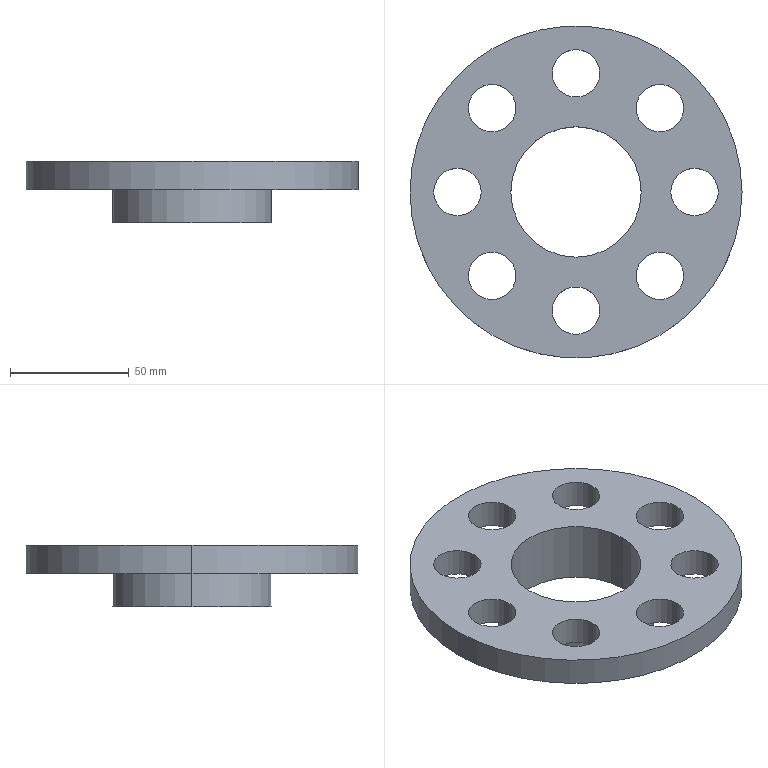Part | SolidWorks | features CirPattern 1, Cut 1, Extrusion 1, ICE 1 | 1 solid | 25 faces | box 140 x 140 x 26 mm | volume 142154 mm3 | cylinder 22 | plane 3 | commonest cylinder face diameters 20 x16 55 x2 67 x2 140 x2
STEP:
#1=CARTESIAN_POINT('',(-33.5,0.,-14.));
#2=VERTEX_POINT('',#1);
#3=CARTESIAN_POINT('',(33.5,0.,-14.));
#4=VERTEX_POINT('',#3);
#5=CARTESIAN_POINT('',(0.,0.,-14.));
#6=DIRECTION('',(0.,0.,-1.));
#7=DIRECTION('',(-1.,0.,0.));
#8=AXIS2_PLACEMENT_3D('',#5,#6,#7);
#9=CIRCLE('',#8,33.5);
#10=EDGE_CURVE('',#2,#4,#9,.T.);
#11=ORIENTED_EDGE('',*,*,#10,.F.);
#12=CARTESIAN_POINT('',(-33.5,0.,0.));
#13=VERTEX_POINT('',#12);
#14=CARTESIAN_POINT('',(-33.5,0.,-14.));
#15=DIRECTION('',(0.,0.,1.));
#16=VECTOR('',#15,1000.);
#17=LINE('',#14,#16);
#18=EDGE_CURVE('',#2,#13,#17,.T.);
#19=ORIENTED_EDGE('',*,*,#18,.T.);
#20=CARTESIAN_POINT('',(33.5,0.,0.));
#21=VERTEX_POINT('',#20);
#22=CARTESIAN_POINT('',(0.,0.,0.));
#23=DIRECTION('',(0.,0.,-1.));
#24=DIRECTION('',(1.,0.,0.));
#25=AXIS2_PLACEMENT_3D('',#22,#23,#24);
#26=CIRCLE('',#25,33.5);
#27=EDGE_CURVE('',#13,#21,#26,.T.);
#28=ORIENTED_EDGE('',*,*,#27,.T.);
#29=CARTESIAN_POINT('',(33.5,0.,-14.));
#30=DIRECTION('',(0.,0.,1.));
#31=VECTOR('',#30,1000.);
#32=LINE('',#29,#31);
#33=EDGE_CURVE('',#4,#21,#32,.T.);
#34=ORIENTED_EDGE('',*,*,#33,.F.);
#35=EDGE_LOOP('',(#11,#19,#28,#34));
#36=FACE_OUTER_BOUND('',#35,.T.);
#37=CARTESIAN_POINT('',(0.,0.,-14.));
#38=DIRECTION('',(0.,0.,1.));
#39=DIRECTION('',(1.,0.,0.));
#40=AXIS2_PLACEMENT_3D('',#37,#38,#39);
#41=CYLINDRICAL_SURFACE('',#40,33.5);
#42=ADVANCED_FACE('',(#36),#41,.T.);
#43=CARTESIAN_POINT('',(40.,0.,0.));
#44=VERTEX_POINT('',#43);
#45=CARTESIAN_POINT('',(60.,0.,0.));
#46=VERTEX_POINT('',#45);
#47=CARTESIAN_POINT('',(50.,0.,0.));
#48=DIRECTION('',(0.,0.,1.));
#49=DIRECTION('',(0.,1.,0.));
#50=AXIS2_PLACEMENT_3D('',#47,#48,#49);
#51=CIRCLE('',#50,10.);
#52=EDGE_CURVE('',#44,#46,#51,.T.);
#53=ORIENTED_EDGE('',*,*,#52,.F.);
#54=CARTESIAN_POINT('',(40.,0.,12.));
#55=VERTEX_POINT('',#54);
#56=CARTESIAN_POINT('',(40.,0.,0.));
#57=DIRECTION('',(0.,0.,1.));
#58=VECTOR('',#57,1000.);
#59=LINE('',#56,#58);
#60=EDGE_CURVE('',#44,#55,#59,.T.);
#61=ORIENTED_EDGE('',*,*,#60,.T.);
#62=CARTESIAN_POINT('',(60.,0.,12.));
#63=VERTEX_POINT('',#62);
#64=CARTESIAN_POINT('',(50.,0.,12.));
#65=DIRECTION('',(0.,0.,1.));
#66=DIRECTION('',(1.,0.,0.));
#67=AXIS2_PLACEMENT_3D('',#64,#65,#66);
#68=CIRCLE('',#67,10.);
#69=EDGE_CURVE('',#55,#63,#68,.T.);
#70=ORIENTED_EDGE('',*,*,#69,.T.);
#71=CARTESIAN_POINT('',(60.,0.,0.));
#72=DIRECTION('',(0.,0.,1.));
#73=VECTOR('',#72,1000.);
#74=LINE('',#71,#73);
#75=EDGE_CURVE('',#46,#63,#74,.T.);
#76=ORIENTED_EDGE('',*,*,#75,.F.);
#77=EDGE_LOOP('',(#53,#61,#70,#76));
#78=FACE_OUTER_BOUND('',#77,.T.);
#79=CARTESIAN_POINT('',(50.,0.,0.));
#80=DIRECTION('',(0.,0.,1.));
#81=DIRECTION('',(1.,0.,0.));
#82=AXIS2_PLACEMENT_3D('',#79,#80,#81);
#83=CYLINDRICAL_SURFACE('',#82,10.);
#84=ADVANCED_FACE('',(#78),#83,.F.);
#85=CARTESIAN_POINT('',(25.355,35.355,0.));
#86=VERTEX_POINT('',#85);
#87=CARTESIAN_POINT('',(45.355,35.355,0.));
#88=VERTEX_POINT('',#87);
#89=CARTESIAN_POINT('',(35.355,35.355,0.));
#90=DIRECTION('',(0.,0.,1.));
#91=DIRECTION('',(-0.7071,0.7071,0.));
#92=AXIS2_PLACEMENT_3D('',#89,#90,#91);
#93=CIRCLE('',#92,10.);
#94=EDGE_CURVE('',#86,#88,#93,.T.);
#95=ORIENTED_EDGE('',*,*,#94,.F.);
#96=CARTESIAN_POINT('',(25.355,35.355,12.));
#97=VERTEX_POINT('',#96);
#98=CARTESIAN_POINT('',(25.355,35.355,0.));
#99=DIRECTION('',(0.,0.,1.));
#100=VECTOR('',#99,1000.);
#101=LINE('',#98,#100);
#102=EDGE_CURVE('',#86,#97,#101,.T.);
#103=ORIENTED_EDGE('',*,*,#102,.T.);
#104=CARTESIAN_POINT('',(45.355,35.355,12.));
#105=VERTEX_POINT('',#104);
#106=CARTESIAN_POINT('',(35.355,35.355,12.));
#107=DIRECTION('',(0.,0.,1.));
#108=DIRECTION('',(1.,0.,0.));
#109=AXIS2_PLACEMENT_3D('',#106,#107,#108);
#110=CIRCLE('',#109,10.);
#111=EDGE_CURVE('',#97,#105,#110,.T.);
#112=ORIENTED_EDGE('',*,*,#111,.T.);
#113=CARTESIAN_POINT('',(45.355,35.355,0.));
#114=DIRECTION('',(0.,0.,1.));
#115=VECTOR('',#114,1000.);
#116=LINE('',#113,#115);
#117=EDGE_CURVE('',#88,#105,#116,.T.);
#118=ORIENTED_EDGE('',*,*,#117,.F.);
#119=EDGE_LOOP('',(#95,#103,#112,#118));
#120=FACE_OUTER_BOUND('',#119,.T.);
#121=CARTESIAN_POINT('',(35.355,35.355,0.));
#122=DIRECTION('',(0.,0.,1.));
#123=DIRECTION('',(1.,0.,0.));
#124=AXIS2_PLACEMENT_3D('',#121,#122,#123);
#125=CYLINDRICAL_SURFACE('',#124,10.);
#126=ADVANCED_FACE('',(#120),#125,.F.);
#127=CARTESIAN_POINT('',(-10.,50.,0.));
#128=VERTEX_POINT('',#127);
#129=CARTESIAN_POINT('',(10.,50.,0.));
#130=VERTEX_POINT('',#129);
#131=CARTESIAN_POINT('',(0.,50.,0.));
#132=DIRECTION('',(0.,0.,1.));
#133=DIRECTION('',(-1.,0.,0.));
#134=AXIS2_PLACEMENT_3D('',#131,#132,#133);
#135=CIRCLE('',#134,10.);
#136=EDGE_CURVE('',#128,#130,#135,.T.);
#137=ORIENTED_EDGE('',*,*,#136,.F.);
#138=CARTESIAN_POINT('',(-10.,50.,12.));
#139=VERTEX_POINT('',#138);
#140=CARTESIAN_POINT('',(-10.,50.,0.));
#141=DIRECTION('',(0.,0.,1.));
#142=VECTOR('',#141,1000.);
#143=LINE('',#140,#142);
#144=EDGE_CURVE('',#128,#139,#143,.T.);
#145=ORIENTED_EDGE('',*,*,#144,.T.);
#146=CARTESIAN_POINT('',(10.,50.,12.));
#147=VERTEX_POINT('',#146);
#148=CARTESIAN_POINT('',(0.,50.,12.));
#149=DIRECTION('',(0.,0.,1.));
#150=DIRECTION('',(1.,0.,0.));
#151=AXIS2_PLACEMENT_3D('',#148,#149,#150);
#152=CIRCLE('',#151,10.);
#153=EDGE_CURVE('',#139,#147,#152,.T.);
#154=ORIENTED_EDGE('',*,*,#153,.T.);
#155=CARTESIAN_POINT('',(10.,50.,0.));
#156=DIRECTION('',(0.,0.,1.));
#157=VECTOR('',#156,1000.);
#158=LINE('',#155,#157);
#159=EDGE_CURVE('',#130,#147,#158,.T.);
#160=ORIENTED_EDGE('',*,*,#159,.F.);
#161=EDGE_LOOP('',(#137,#145,#154,#160));
#162=FACE_OUTER_BOUND('',#161,.T.);
#163=CARTESIAN_POINT('',(0.,50.,0.));
#164=DIRECTION('',(0.,0.,1.));
#165=DIRECTION('',(1.,0.,0.));
#166=AXIS2_PLACEMENT_3D('',#163,#164,#165);
#167=CYLINDRICAL_SURFACE('',#166,10.);
#168=ADVANCED_FACE('',(#162),#167,.F.);
#169=CARTESIAN_POINT('',(-45.355,35.355,0.));
#170=VERTEX_POINT('',#169);
#171=CARTESIAN_POINT('',(-25.355,35.355,0.));
#172=VERTEX_POINT('',#171);
#173=CARTESIAN_POINT('',(-35.355,35.355,0.));
#174=DIRECTION('',(0.,0.,1.));
#175=DIRECTION('',(-0.7071,-0.7071,0.));
#176=AXIS2_PLACEMENT_3D('',#173,#174,#175);
#177=CIRCLE('',#176,10.);
#178=EDGE_CURVE('',#170,#172,#177,.T.);
#179=ORIENTED_EDGE('',*,*,#178,.F.);
#180=CARTESIAN_POINT('',(-45.355,35.355,12.));
#181=VERTEX_POINT('',#180);
#182=CARTESIAN_POINT('',(-45.355,35.355,0.));
#183=DIRECTION('',(0.,0.,1.));
#184=VECTOR('',#183,1000.);
#185=LINE('',#182,#184);
#186=EDGE_CURVE('',#170,#181,#185,.T.);
#187=ORIENTED_EDGE('',*,*,#186,.T.);
#188=CARTESIAN_POINT('',(-25.355,35.355,12.));
#189=VERTEX_POINT('',#188);
#190=CARTESIAN_POINT('',(-35.355,35.355,12.));
#191=DIRECTION('',(0.,0.,1.));
#192=DIRECTION('',(1.,0.,0.));
#193=AXIS2_PLACEMENT_3D('',#190,#191,#192);
#194=CIRCLE('',#193,10.);
#195=EDGE_CURVE('',#181,#189,#194,.T.);
#196=ORIENTED_EDGE('',*,*,#195,.T.);
#197=CARTESIAN_POINT('',(-25.355,35.355,0.));
#198=DIRECTION('',(0.,0.,1.));
#199=VECTOR('',#198,1000.);
#200=LINE('',#197,#199);
#201=EDGE_CURVE('',#172,#189,#200,.T.);
#202=ORIENTED_EDGE('',*,*,#201,.F.);
#203=EDGE_LOOP('',(#179,#187,#196,#202));
#204=FACE_OUTER_BOUND('',#203,.T.);
#205=CARTESIAN_POINT('',(-35.355,35.355,0.));
#206=DIRECTION('',(0.,0.,1.));
#207=DIRECTION('',(1.,0.,0.));
#208=AXIS2_PLACEMENT_3D('',#205,#206,#207);
#209=CYLINDRICAL_SURFACE('',#208,10.);
#210=ADVANCED_FACE('',(#204),#209,.F.);
#211=CARTESIAN_POINT('',(-60.,0.,0.));
#212=VERTEX_POINT('',#211);
#213=CARTESIAN_POINT('',(-40.,0.,0.));
#214=VERTEX_POINT('',#213);
#215=CARTESIAN_POINT('',(-50.,0.,0.));
#216=DIRECTION('',(0.,0.,1.));
#217=DIRECTION('',(0.,-1.,0.));
#218=AXIS2_PLACEMENT_3D('',#215,#216,#217);
#219=CIRCLE('',#218,10.);
#220=EDGE_CURVE('',#212,#214,#219,.T.);
#221=ORIENTED_EDGE('',*,*,#220,.F.);
#222=CARTESIAN_POINT('',(-60.,0.,12.));
#223=VERTEX_POINT('',#222);
#224=CARTESIAN_POINT('',(-60.,0.,0.));
#225=DIRECTION('',(0.,0.,1.));
#226=VECTOR('',#225,1000.);
#227=LINE('',#224,#226);
#228=EDGE_CURVE('',#212,#223,#227,.T.);
#229=ORIENTED_EDGE('',*,*,#228,.T.);
#230=CARTESIAN_POINT('',(-40.,0.,12.));
#231=VERTEX_POINT('',#230);
#232=CARTESIAN_POINT('',(-50.,0.,12.));
#233=DIRECTION('',(0.,0.,1.));
#234=DIRECTION('',(1.,0.,0.));
#235=AXIS2_PLACEMENT_3D('',#232,#233,#234);
#236=CIRCLE('',#235,10.);
#237=EDGE_CURVE('',#223,#231,#236,.T.);
#238=ORIENTED_EDGE('',*,*,#237,.T.);
#239=CARTESIAN_POINT('',(-40.,0.,0.));
#240=DIRECTION('',(0.,0.,1.));
#241=VECTOR('',#240,1000.);
#242=LINE('',#239,#241);
#243=EDGE_CURVE('',#214,#231,#242,.T.);
#244=ORIENTED_EDGE('',*,*,#243,.F.);
#245=EDGE_LOOP('',(#221,#229,#238,#244));
#246=FACE_OUTER_BOUND('',#245,.T.);
#247=CARTESIAN_POINT('',(-50.,0.,0.));
#248=DIRECTION('',(0.,0.,1.));
#249=DIRECTION('',(1.,0.,0.));
#250=AXIS2_PLACEMENT_3D('',#247,#248,#249);
#251=CYLINDRICAL_SURFACE('',#250,10.);
#252=ADVANCED_FACE('',(#246),#251,.F.);
#253=CARTESIAN_POINT('',(-45.355,-35.355,0.));
#254=VERTEX_POINT('',#253);
#255=CARTESIAN_POINT('',(-25.355,-35.355,0.));
#256=VERTEX_POINT('',#255);
#257=CARTESIAN_POINT('',(-35.355,-35.355,0.));
#258=DIRECTION('',(0.,0.,1.));
#259=DIRECTION('',(0.7071,-0.7071,0.));
#260=AXIS2_PLACEMENT_3D('',#257,#258,#259);
#261=CIRCLE('',#260,10.);
#262=EDGE_CURVE('',#254,#256,#261,.T.);
#263=ORIENTED_EDGE('',*,*,#262,.F.);
#264=CARTESIAN_POINT('',(-45.355,-35.355,12.));
#265=VERTEX_POINT('',#264);
#266=CARTESIAN_POINT('',(-45.355,-35.355,0.));
#267=DIRECTION('',(0.,0.,1.));
#268=VECTOR('',#267,1000.);
#269=LINE('',#266,#268);
#270=EDGE_CURVE('',#254,#265,#269,.T.);
#271=ORIENTED_EDGE('',*,*,#270,.T.);
#272=CARTESIAN_POINT('',(-25.355,-35.355,12.));
#273=VERTEX_POINT('',#272);
#274=CARTESIAN_POINT('',(-35.355,-35.355,12.));
#275=DIRECTION('',(0.,0.,1.));
#276=DIRECTION('',(1.,0.,0.));
#277=AXIS2_PLACEMENT_3D('',#274,#275,#276);
#278=CIRCLE('',#277,10.);
#279=EDGE_CURVE('',#265,#273,#278,.T.);
#280=ORIENTED_EDGE('',*,*,#279,.T.);
#281=CARTESIAN_POINT('',(-25.355,-35.355,0.));
#282=DIRECTION('',(0.,0.,1.));
#283=VECTOR('',#282,1000.);
#284=LINE('',#281,#283);
#285=EDGE_CURVE('',#256,#273,#284,.T.);
#286=ORIENTED_EDGE('',*,*,#285,.F.);
#287=EDGE_LOOP('',(#263,#271,#280,#286));
#288=FACE_OUTER_BOUND('',#287,.T.);
#289=CARTESIAN_POINT('',(-35.355,-35.355,0.));
#290=DIRECTION('',(0.,0.,1.));
#291=DIRECTION('',(1.,0.,0.));
#292=AXIS2_PLACEMENT_3D('',#289,#290,#291);
#293=CYLINDRICAL_SURFACE('',#292,10.);
#294=ADVANCED_FACE('',(#288),#293,.F.);
#295=CARTESIAN_POINT('',(25.355,-35.355,0.));
#296=VERTEX_POINT('',#295);
#297=CARTESIAN_POINT('',(45.355,-35.355,0.));
#298=VERTEX_POINT('',#297);
#299=CARTESIAN_POINT('',(35.355,-35.355,0.));
#300=DIRECTION('',(0.,0.,1.));
#301=DIRECTION('',(0.7071,0.7071,0.));
#302=AXIS2_PLACEMENT_3D('',#299,#300,#301);
#303=CIRCLE('',#302,10.);
#304=EDGE_CURVE('',#296,#298,#303,.T.);
#305=ORIENTED_EDGE('',*,*,#304,.F.);
#306=CARTESIAN_POINT('',(25.355,-35.355,12.));
#307=VERTEX_POINT('',#306);
#308=CARTESIAN_POINT('',(25.355,-35.355,0.));
#309=DIRECTION('',(0.,0.,1.));
#310=VECTOR('',#309,1000.);
#311=LINE('',#308,#310);
#312=EDGE_CURVE('',#296,#307,#311,.T.);
#313=ORIENTED_EDGE('',*,*,#312,.T.);
#314=CARTESIAN_POINT('',(45.355,-35.355,12.));
#315=VERTEX_POINT('',#314);
#316=CARTESIAN_POINT('',(35.355,-35.355,12.));
#317=DIRECTION('',(0.,0.,1.));
#318=DIRECTION('',(1.,0.,0.));
#319=AXIS2_PLACEMENT_3D('',#316,#317,#318);
#320=CIRCLE('',#319,10.);
#321=EDGE_CURVE('',#307,#315,#320,.T.);
#322=ORIENTED_EDGE('',*,*,#321,.T.);
#323=CARTESIAN_POINT('',(45.355,-35.355,0.));
#324=DIRECTION('',(0.,0.,1.));
#325=VECTOR('',#324,1000.);
#326=LINE('',#323,#325);
#327=EDGE_CURVE('',#298,#315,#326,.T.);
#328=ORIENTED_EDGE('',*,*,#327,.F.);
#329=EDGE_LOOP('',(#305,#313,#322,#328));
#330=FACE_OUTER_BOUND('',#329,.T.);
#331=CARTESIAN_POINT('',(35.355,-35.355,0.));
#332=DIRECTION('',(0.,0.,1.));
#333=DIRECTION('',(1.,0.,0.));
#334=AXIS2_PLACEMENT_3D('',#331,#332,#333);
#335=CYLINDRICAL_SURFACE('',#334,10.);
#336=ADVANCED_FACE('',(#330),#335,.F.);
#337=CARTESIAN_POINT('',(-10.,-50.,0.));
#338=VERTEX_POINT('',#337);
#339=CARTESIAN_POINT('',(10.,-50.,0.));
#340=VERTEX_POINT('',#339);
#341=CARTESIAN_POINT('',(0.,-50.,0.));
#342=DIRECTION('',(0.,0.,1.));
#343=DIRECTION('',(1.,0.,0.));
#344=AXIS2_PLACEMENT_3D('',#341,#342,#343);
#345=CIRCLE('',#344,10.);
#346=EDGE_CURVE('',#338,#340,#345,.T.);
#347=ORIENTED_EDGE('',*,*,#346,.F.);
#348=CARTESIAN_POINT('',(-10.,-50.,12.));
#349=VERTEX_POINT('',#348);
#350=CARTESIAN_POINT('',(-10.,-50.,0.));
#351=DIRECTION('',(0.,0.,1.));
#352=VECTOR('',#351,1000.);
#353=LINE('',#350,#352);
#354=EDGE_CURVE('',#338,#349,#353,.T.);
#355=ORIENTED_EDGE('',*,*,#354,.T.);
#356=CARTESIAN_POINT('',(10.,-50.,12.));
#357=VERTEX_POINT('',#356);
#358=CARTESIAN_POINT('',(0.,-50.,12.));
#359=DIRECTION('',(0.,0.,1.));
#360=DIRECTION('',(1.,0.,0.));
#361=AXIS2_PLACEMENT_3D('',#358,#359,#360);
#362=CIRCLE('',#361,10.);
#363=EDGE_CURVE('',#349,#357,#362,.T.);
#364=ORIENTED_EDGE('',*,*,#363,.T.);
#365=CARTESIAN_POINT('',(10.,-50.,0.));
#366=DIRECTION('',(0.,0.,1.));
#367=VECTOR('',#366,1000.);
#368=LINE('',#365,#367);
#369=EDGE_CURVE('',#340,#357,#368,.T.);
#370=ORIENTED_EDGE('',*,*,#369,.F.);
#371=EDGE_LOOP('',(#347,#355,#364,#370));
#372=FACE_OUTER_BOUND('',#371,.T.);
#373=CARTESIAN_POINT('',(0.,-50.,0.));
#374=DIRECTION('',(0.,0.,1.));
#375=DIRECTION('',(1.,0.,0.));
#376=AXIS2_PLACEMENT_3D('',#373,#374,#375);
#377=CYLINDRICAL_SURFACE('',#376,10.);
#378=ADVANCED_FACE('',(#372),#377,.F.);
#379=CARTESIAN_POINT('',(-27.5,0.,12.));
#380=VERTEX_POINT('',#379);
#381=CARTESIAN_POINT('',(27.5,0.,12.));
#382=VERTEX_POINT('',#381);
#383=CARTESIAN_POINT('',(0.,0.,12.));
#384=DIRECTION('',(0.,0.,1.));
#385=DIRECTION('',(1.,0.,0.));
#386=AXIS2_PLACEMENT_3D('',#383,#384,#385);
#387=CIRCLE('',#386,27.5);
#388=EDGE_CURVE('',#380,#382,#387,.T.);
#389=ORIENTED_EDGE('',*,*,#388,.T.);
#390=CARTESIAN_POINT('',(27.5,0.,-14.));
#391=VERTEX_POINT('',#390);
#392=CARTESIAN_POINT('',(27.5,0.,12.));
#393=DIRECTION('',(0.,0.,-1.));
#394=VECTOR('',#393,1000.);
#395=LINE('',#392,#394);
#396=EDGE_CURVE('',#382,#391,#395,.T.);
#397=ORIENTED_EDGE('',*,*,#396,.T.);
#398=CARTESIAN_POINT('',(-27.5,0.,-14.));
#399=VERTEX_POINT('',#398);
#400=CARTESIAN_POINT('',(0.,0.,-14.));
#401=DIRECTION('',(0.,0.,-1.));
#402=DIRECTION('',(-1.,0.,0.));
#403=AXIS2_PLACEMENT_3D('',#400,#401,#402);
#404=CIRCLE('',#403,27.5);
#405=EDGE_CURVE('',#391,#399,#404,.T.);
#406=ORIENTED_EDGE('',*,*,#405,.T.);
#407=CARTESIAN_POINT('',(-27.5,0.,12.));
#408=DIRECTION('',(0.,0.,-1.));
#409=VECTOR('',#408,1000.);
#410=LINE('',#407,#409);
#411=EDGE_CURVE('',#380,#399,#410,.T.);
#412=ORIENTED_EDGE('',*,*,#411,.F.);
#413=EDGE_LOOP('',(#389,#397,#406,#412));
#414=FACE_OUTER_BOUND('',#413,.T.);
#415=CARTESIAN_POINT('',(0.,0.,12.));
#416=DIRECTION('',(0.,0.,-1.));
#417=DIRECTION('',(-1.,0.,0.));
#418=AXIS2_PLACEMENT_3D('',#415,#416,#417);
#419=CYLINDRICAL_SURFACE('',#418,27.5);
#420=ADVANCED_FACE('',(#414),#419,.F.);
#421=CARTESIAN_POINT('',(70.,0.,12.));
#422=VERTEX_POINT('',#421);
#423=CARTESIAN_POINT('',(-70.,0.,12.));
#424=VERTEX_POINT('',#423);
#425=CARTESIAN_POINT('',(0.,0.,12.));
#426=DIRECTION('',(0.,0.,1.));
#427=DIRECTION('',(1.,0.,0.));
#428=AXIS2_PLACEMENT_3D('',#425,#426,#427);
#429=CIRCLE('',#428,70.);
#430=EDGE_CURVE('',#422,#424,#429,.T.);
#431=ORIENTED_EDGE('',*,*,#430,.F.);
#432=CARTESIAN_POINT('',(70.,0.,0.));
#433=VERTEX_POINT('',#432);
#434=CARTESIAN_POINT('',(70.,0.,12.));
#435=DIRECTION('',(0.,0.,-1.));
#436=VECTOR('',#435,1000.);
#437=LINE('',#434,#436);
#438=EDGE_CURVE('',#422,#433,#437,.T.);
#439=ORIENTED_EDGE('',*,*,#438,.T.);
#440=CARTESIAN_POINT('',(-70.,0.,0.));
#441=VERTEX_POINT('',#440);
#442=CARTESIAN_POINT('',(0.,0.,0.));
#443=DIRECTION('',(0.,0.,1.));
#444=DIRECTION('',(1.,0.,0.));
#445=AXIS2_PLACEMENT_3D('',#442,#443,#444);
#446=CIRCLE('',#445,70.);
#447=EDGE_CURVE('',#433,#441,#446,.T.);
#448=ORIENTED_EDGE('',*,*,#447,.T.);
#449=CARTESIAN_POINT('',(-70.,0.,12.));
#450=DIRECTION('',(0.,0.,-1.));
#451=VECTOR('',#450,1000.);
#452=LINE('',#449,#451);
#453=EDGE_CURVE('',#424,#441,#452,.T.);
#454=ORIENTED_EDGE('',*,*,#453,.F.);
#455=EDGE_LOOP('',(#431,#439,#448,#454));
#456=FACE_OUTER_BOUND('',#455,.T.);
#457=CARTESIAN_POINT('',(0.,0.,12.));
#458=DIRECTION('',(0.,0.,-1.));
#459=DIRECTION('',(-1.,0.,0.));
#460=AXIS2_PLACEMENT_3D('',#457,#458,#459);
#461=CYLINDRICAL_SURFACE('',#460,70.);
#462=ADVANCED_FACE('',(#456),#461,.T.);
#463=CARTESIAN_POINT('',(0.,0.,0.));
#464=DIRECTION('',(0.,0.,1.));
#465=DIRECTION('',(1.,0.,0.));
#466=AXIS2_PLACEMENT_3D('',#463,#464,#465);
#467=CIRCLE('',#466,70.);
#468=EDGE_CURVE('',#441,#433,#467,.T.);
#469=ORIENTED_EDGE('',*,*,#468,.F.);
#470=ORIENTED_EDGE('',*,*,#447,.F.);
#471=EDGE_LOOP('',(#469,#470));
#472=FACE_OUTER_BOUND('',#471,.T.);
#473=CARTESIAN_POINT('',(0.,-50.,0.));
#474=DIRECTION('',(0.,0.,1.));
#475=DIRECTION('',(1.,0.,0.));
#476=AXIS2_PLACEMENT_3D('',#473,#474,#475);
#477=CIRCLE('',#476,10.);
#478=EDGE_CURVE('',#340,#338,#477,.T.);
#479=ORIENTED_EDGE('',*,*,#478,.T.);
#480=ORIENTED_EDGE('',*,*,#346,.T.);
#481=EDGE_LOOP('',(#479,#480));
#482=FACE_BOUND('',#481,.T.);
#483=CARTESIAN_POINT('',(35.355,-35.355,0.));
#484=DIRECTION('',(0.,0.,1.));
#485=DIRECTION('',(0.7071,0.7071,0.));
#486=AXIS2_PLACEMENT_3D('',#483,#484,#485);
#487=CIRCLE('',#486,10.);
#488=EDGE_CURVE('',#298,#296,#487,.T.);
#489=ORIENTED_EDGE('',*,*,#488,.T.);
#490=ORIENTED_EDGE('',*,*,#304,.T.);
#491=EDGE_LOOP('',(#489,#490));
#492=FACE_BOUND('',#491,.T.);
#493=CARTESIAN_POINT('',(-35.355,-35.355,0.));
#494=DIRECTION('',(0.,0.,1.));
#495=DIRECTION('',(0.7071,-0.7071,0.));
#496=AXIS2_PLACEMENT_3D('',#493,#494,#495);
#497=CIRCLE('',#496,10.);
#498=EDGE_CURVE('',#256,#254,#497,.T.);
#499=ORIENTED_EDGE('',*,*,#498,.T.);
#500=ORIENTED_EDGE('',*,*,#262,.T.);
#501=EDGE_LOOP('',(#499,#500));
#502=FACE_BOUND('',#501,.T.);
#503=CARTESIAN_POINT('',(-50.,0.,0.));
#504=DIRECTION('',(0.,0.,1.));
#505=DIRECTION('',(0.,-1.,0.));
#506=AXIS2_PLACEMENT_3D('',#503,#504,#505);
#507=CIRCLE('',#506,10.);
#508=EDGE_CURVE('',#214,#212,#507,.T.);
#509=ORIENTED_EDGE('',*,*,#508,.T.);
#510=ORIENTED_EDGE('',*,*,#220,.T.);
#511=EDGE_LOOP('',(#509,#510));
#512=FACE_BOUND('',#511,.T.);
#513=CARTESIAN_POINT('',(-35.355,35.355,0.));
#514=DIRECTION('',(0.,0.,1.));
#515=DIRECTION('',(-0.7071,-0.7071,0.));
#516=AXIS2_PLACEMENT_3D('',#513,#514,#515);
#517=CIRCLE('',#516,10.);
#518=EDGE_CURVE('',#172,#170,#517,.T.);
#519=ORIENTED_EDGE('',*,*,#518,.T.);
#520=ORIENTED_EDGE('',*,*,#178,.T.);
#521=EDGE_LOOP('',(#519,#520));
#522=FACE_BOUND('',#521,.T.);
#523=CARTESIAN_POINT('',(0.,50.,0.));
#524=DIRECTION('',(0.,0.,1.));
#525=DIRECTION('',(-1.,0.,0.));
#526=AXIS2_PLACEMENT_3D('',#523,#524,#525);
#527=CIRCLE('',#526,10.);
#528=EDGE_CURVE('',#130,#128,#527,.T.);
#529=ORIENTED_EDGE('',*,*,#528,.T.);
#530=ORIENTED_EDGE('',*,*,#136,.T.);
#531=EDGE_LOOP('',(#529,#530));
#532=FACE_BOUND('',#531,.T.);
#533=CARTESIAN_POINT('',(35.355,35.355,0.));
#534=DIRECTION('',(0.,0.,1.));
#535=DIRECTION('',(-0.7071,0.7071,0.));
#536=AXIS2_PLACEMENT_3D('',#533,#534,#535);
#537=CIRCLE('',#536,10.);
#538=EDGE_CURVE('',#88,#86,#537,.T.);
#539=ORIENTED_EDGE('',*,*,#538,.T.);
#540=ORIENTED_EDGE('',*,*,#94,.T.);
#541=EDGE_LOOP('',(#539,#540));
#542=FACE_BOUND('',#541,.T.);
#543=CARTESIAN_POINT('',(50.,0.,0.));
#544=DIRECTION('',(0.,0.,1.));
#545=DIRECTION('',(0.,1.,0.));
#546=AXIS2_PLACEMENT_3D('',#543,#544,#545);
#547=CIRCLE('',#546,10.);
#548=EDGE_CURVE('',#46,#44,#547,.T.);
#549=ORIENTED_EDGE('',*,*,#548,.T.);
#550=ORIENTED_EDGE('',*,*,#52,.T.);
#551=EDGE_LOOP('',(#549,#550));
#552=FACE_BOUND('',#551,.T.);
#553=CARTESIAN_POINT('',(0.,0.,0.));
#554=DIRECTION('',(0.,0.,-1.));
#555=DIRECTION('',(1.,0.,0.));
#556=AXIS2_PLACEMENT_3D('',#553,#554,#555);
#557=CIRCLE('',#556,33.5);
#558=EDGE_CURVE('',#21,#13,#557,.T.);
#559=ORIENTED_EDGE('',*,*,#558,.F.);
#560=ORIENTED_EDGE('',*,*,#27,.F.);
#561=EDGE_LOOP('',(#559,#560));
#562=FACE_BOUND('',#561,.T.);
#563=CARTESIAN_POINT('',(0.,0.,0.));
#564=DIRECTION('',(0.,0.,1.));
#565=DIRECTION('',(1.,0.,0.));
#566=AXIS2_PLACEMENT_3D('',#563,#564,#565);
#567=PLANE('',#566);
#568=ADVANCED_FACE('',(#472,#482,#492,#502,#512,#522,#532,#542,#552,#562),#567,.F.);
#569=CARTESIAN_POINT('',(50.,0.,12.));
#570=DIRECTION('',(0.,0.,1.));
#571=DIRECTION('',(1.,0.,0.));
#572=AXIS2_PLACEMENT_3D('',#569,#570,#571);
#573=CIRCLE('',#572,10.);
#574=EDGE_CURVE('',#63,#55,#573,.T.);
#575=ORIENTED_EDGE('',*,*,#574,.F.);
#576=ORIENTED_EDGE('',*,*,#69,.F.);
#577=EDGE_LOOP('',(#575,#576));
#578=FACE_BOUND('',#577,.T.);
#579=CARTESIAN_POINT('',(35.355,35.355,12.));
#580=DIRECTION('',(0.,0.,1.));
#581=DIRECTION('',(1.,0.,0.));
#582=AXIS2_PLACEMENT_3D('',#579,#580,#581);
#583=CIRCLE('',#582,10.);
#584=EDGE_CURVE('',#105,#97,#583,.T.);
#585=ORIENTED_EDGE('',*,*,#584,.F.);
#586=ORIENTED_EDGE('',*,*,#111,.F.);
#587=EDGE_LOOP('',(#585,#586));
#588=FACE_BOUND('',#587,.T.);
#589=CARTESIAN_POINT('',(0.,50.,12.));
#590=DIRECTION('',(0.,0.,1.));
#591=DIRECTION('',(1.,0.,0.));
#592=AXIS2_PLACEMENT_3D('',#589,#590,#591);
#593=CIRCLE('',#592,10.);
#594=EDGE_CURVE('',#147,#139,#593,.T.);
#595=ORIENTED_EDGE('',*,*,#594,.F.);
#596=ORIENTED_EDGE('',*,*,#153,.F.);
#597=EDGE_LOOP('',(#595,#596));
#598=FACE_BOUND('',#597,.T.);
#599=CARTESIAN_POINT('',(-35.355,35.355,12.));
#600=DIRECTION('',(0.,0.,1.));
#601=DIRECTION('',(1.,0.,0.));
#602=AXIS2_PLACEMENT_3D('',#599,#600,#601);
#603=CIRCLE('',#602,10.);
#604=EDGE_CURVE('',#189,#181,#603,.T.);
#605=ORIENTED_EDGE('',*,*,#604,.F.);
#606=ORIENTED_EDGE('',*,*,#195,.F.);
#607=EDGE_LOOP('',(#605,#606));
#608=FACE_BOUND('',#607,.T.);
#609=CARTESIAN_POINT('',(-50.,0.,12.));
#610=DIRECTION('',(0.,0.,1.));
#611=DIRECTION('',(1.,0.,0.));
#612=AXIS2_PLACEMENT_3D('',#609,#610,#611);
#613=CIRCLE('',#612,10.);
#614=EDGE_CURVE('',#231,#223,#613,.T.);
#615=ORIENTED_EDGE('',*,*,#614,.F.);
#616=ORIENTED_EDGE('',*,*,#237,.F.);
#617=EDGE_LOOP('',(#615,#616));
#618=FACE_BOUND('',#617,.T.);
#619=CARTESIAN_POINT('',(-35.355,-35.355,12.));
#620=DIRECTION('',(0.,0.,1.));
#621=DIRECTION('',(1.,0.,0.));
#622=AXIS2_PLACEMENT_3D('',#619,#620,#621);
#623=CIRCLE('',#622,10.);
#624=EDGE_CURVE('',#273,#265,#623,.T.);
#625=ORIENTED_EDGE('',*,*,#624,.F.);
#626=ORIENTED_EDGE('',*,*,#279,.F.);
#627=EDGE_LOOP('',(#625,#626));
#628=FACE_BOUND('',#627,.T.);
#629=CARTESIAN_POINT('',(35.355,-35.355,12.));
#630=DIRECTION('',(0.,0.,1.));
#631=DIRECTION('',(1.,0.,0.));
#632=AXIS2_PLACEMENT_3D('',#629,#630,#631);
#633=CIRCLE('',#632,10.);
#634=EDGE_CURVE('',#315,#307,#633,.T.);
#635=ORIENTED_EDGE('',*,*,#634,.F.);
#636=ORIENTED_EDGE('',*,*,#321,.F.);
#637=EDGE_LOOP('',(#635,#636));
#638=FACE_BOUND('',#637,.T.);
#639=CARTESIAN_POINT('',(0.,-50.,12.));
#640=DIRECTION('',(0.,0.,1.));
#641=DIRECTION('',(1.,0.,0.));
#642=AXIS2_PLACEMENT_3D('',#639,#640,#641);
#643=CIRCLE('',#642,10.);
#644=EDGE_CURVE('',#357,#349,#643,.T.);
#645=ORIENTED_EDGE('',*,*,#644,.F.);
#646=ORIENTED_EDGE('',*,*,#363,.F.);
#647=EDGE_LOOP('',(#645,#646));
#648=FACE_BOUND('',#647,.T.);
#649=CARTESIAN_POINT('',(0.,0.,12.));
#650=DIRECTION('',(0.,0.,1.));
#651=DIRECTION('',(1.,0.,0.));
#652=AXIS2_PLACEMENT_3D('',#649,#650,#651);
#653=CIRCLE('',#652,70.);
#654=EDGE_CURVE('',#424,#422,#653,.T.);
#655=ORIENTED_EDGE('',*,*,#654,.T.);
#656=ORIENTED_EDGE('',*,*,#430,.T.);
#657=EDGE_LOOP('',(#655,#656));
#658=FACE_OUTER_BOUND('',#657,.T.);
#659=ORIENTED_EDGE('',*,*,#388,.F.);
#660=CARTESIAN_POINT('',(0.,0.,12.));
#661=DIRECTION('',(0.,0.,1.));
#662=DIRECTION('',(1.,0.,0.));
#663=AXIS2_PLACEMENT_3D('',#660,#661,#662);
#664=CIRCLE('',#663,27.5);
#665=EDGE_CURVE('',#382,#380,#664,.T.);
#666=ORIENTED_EDGE('',*,*,#665,.F.);
#667=EDGE_LOOP('',(#659,#666));
#668=FACE_BOUND('',#667,.T.);
#669=CARTESIAN_POINT('',(0.,0.,12.));
#670=DIRECTION('',(0.,0.,1.));
#671=DIRECTION('',(1.,0.,0.));
#672=AXIS2_PLACEMENT_3D('',#669,#670,#671);
#673=PLANE('',#672);
#674=ADVANCED_FACE('',(#578,#588,#598,#608,#618,#628,#638,#648,#658,#668),#673,.T.);
#675=ORIENTED_EDGE('',*,*,#438,.F.);
#676=ORIENTED_EDGE('',*,*,#654,.F.);
#677=ORIENTED_EDGE('',*,*,#453,.T.);
#678=ORIENTED_EDGE('',*,*,#468,.T.);
#679=EDGE_LOOP('',(#675,#676,#677,#678));
#680=FACE_OUTER_BOUND('',#679,.T.);
#681=CARTESIAN_POINT('',(0.,0.,12.));
#682=DIRECTION('',(0.,0.,-1.));
#683=DIRECTION('',(-1.,0.,0.));
#684=AXIS2_PLACEMENT_3D('',#681,#682,#683);
#685=CYLINDRICAL_SURFACE('',#684,70.);
#686=ADVANCED_FACE('',(#680),#685,.T.);
#687=ORIENTED_EDGE('',*,*,#396,.F.);
#688=ORIENTED_EDGE('',*,*,#665,.T.);
#689=ORIENTED_EDGE('',*,*,#411,.T.);
#690=CARTESIAN_POINT('',(0.,0.,-14.));
#691=DIRECTION('',(0.,0.,-1.));
#692=DIRECTION('',(-1.,0.,0.));
#693=AXIS2_PLACEMENT_3D('',#690,#691,#692);
#694=CIRCLE('',#693,27.5);
#695=EDGE_CURVE('',#399,#391,#694,.T.);
#696=ORIENTED_EDGE('',*,*,#695,.T.);
#697=EDGE_LOOP('',(#687,#688,#689,#696));
#698=FACE_OUTER_BOUND('',#697,.T.);
#699=CARTESIAN_POINT('',(0.,0.,12.));
#700=DIRECTION('',(0.,0.,-1.));
#701=DIRECTION('',(-1.,0.,0.));
#702=AXIS2_PLACEMENT_3D('',#699,#700,#701);
#703=CYLINDRICAL_SURFACE('',#702,27.5);
#704=ADVANCED_FACE('',(#698),#703,.F.);
#705=ORIENTED_EDGE('',*,*,#354,.F.);
#706=ORIENTED_EDGE('',*,*,#478,.F.);
#707=ORIENTED_EDGE('',*,*,#369,.T.);
#708=ORIENTED_EDGE('',*,*,#644,.T.);
#709=EDGE_LOOP('',(#705,#706,#707,#708));
#710=FACE_OUTER_BOUND('',#709,.T.);
#711=CARTESIAN_POINT('',(0.,-50.,0.));
#712=DIRECTION('',(0.,0.,1.));
#713=DIRECTION('',(1.,0.,0.));
#714=AXIS2_PLACEMENT_3D('',#711,#712,#713);
#715=CYLINDRICAL_SURFACE('',#714,10.);
#716=ADVANCED_FACE('',(#710),#715,.F.);
#717=ORIENTED_EDGE('',*,*,#312,.F.);
#718=ORIENTED_EDGE('',*,*,#488,.F.);
#719=ORIENTED_EDGE('',*,*,#327,.T.);
#720=ORIENTED_EDGE('',*,*,#634,.T.);
#721=EDGE_LOOP('',(#717,#718,#719,#720));
#722=FACE_OUTER_BOUND('',#721,.T.);
#723=CARTESIAN_POINT('',(35.355,-35.355,0.));
#724=DIRECTION('',(0.,0.,1.));
#725=DIRECTION('',(1.,0.,0.));
#726=AXIS2_PLACEMENT_3D('',#723,#724,#725);
#727=CYLINDRICAL_SURFACE('',#726,10.);
#728=ADVANCED_FACE('',(#722),#727,.F.);
#729=ORIENTED_EDGE('',*,*,#270,.F.);
#730=ORIENTED_EDGE('',*,*,#498,.F.);
#731=ORIENTED_EDGE('',*,*,#285,.T.);
#732=ORIENTED_EDGE('',*,*,#624,.T.);
#733=EDGE_LOOP('',(#729,#730,#731,#732));
#734=FACE_OUTER_BOUND('',#733,.T.);
#735=CARTESIAN_POINT('',(-35.355,-35.355,0.));
#736=DIRECTION('',(0.,0.,1.));
#737=DIRECTION('',(1.,0.,0.));
#738=AXIS2_PLACEMENT_3D('',#735,#736,#737);
#739=CYLINDRICAL_SURFACE('',#738,10.);
#740=ADVANCED_FACE('',(#734),#739,.F.);
#741=ORIENTED_EDGE('',*,*,#228,.F.);
#742=ORIENTED_EDGE('',*,*,#508,.F.);
#743=ORIENTED_EDGE('',*,*,#243,.T.);
#744=ORIENTED_EDGE('',*,*,#614,.T.);
#745=EDGE_LOOP('',(#741,#742,#743,#744));
#746=FACE_OUTER_BOUND('',#745,.T.);
#747=CARTESIAN_POINT('',(-50.,0.,0.));
#748=DIRECTION('',(0.,0.,1.));
#749=DIRECTION('',(1.,0.,0.));
#750=AXIS2_PLACEMENT_3D('',#747,#748,#749);
#751=CYLINDRICAL_SURFACE('',#750,10.);
#752=ADVANCED_FACE('',(#746),#751,.F.);
#753=ORIENTED_EDGE('',*,*,#186,.F.);
#754=ORIENTED_EDGE('',*,*,#518,.F.);
#755=ORIENTED_EDGE('',*,*,#201,.T.);
#756=ORIENTED_EDGE('',*,*,#604,.T.);
#757=EDGE_LOOP('',(#753,#754,#755,#756));
#758=FACE_OUTER_BOUND('',#757,.T.);
#759=CARTESIAN_POINT('',(-35.355,35.355,0.));
#760=DIRECTION('',(0.,0.,1.));
#761=DIRECTION('',(1.,0.,0.));
#762=AXIS2_PLACEMENT_3D('',#759,#760,#761);
#763=CYLINDRICAL_SURFACE('',#762,10.);
#764=ADVANCED_FACE('',(#758),#763,.F.);
#765=ORIENTED_EDGE('',*,*,#144,.F.);
#766=ORIENTED_EDGE('',*,*,#528,.F.);
#767=ORIENTED_EDGE('',*,*,#159,.T.);
#768=ORIENTED_EDGE('',*,*,#594,.T.);
#769=EDGE_LOOP('',(#765,#766,#767,#768));
#770=FACE_OUTER_BOUND('',#769,.T.);
#771=CARTESIAN_POINT('',(0.,50.,0.));
#772=DIRECTION('',(0.,0.,1.));
#773=DIRECTION('',(1.,0.,0.));
#774=AXIS2_PLACEMENT_3D('',#771,#772,#773);
#775=CYLINDRICAL_SURFACE('',#774,10.);
#776=ADVANCED_FACE('',(#770),#775,.F.);
#777=ORIENTED_EDGE('',*,*,#102,.F.);
#778=ORIENTED_EDGE('',*,*,#538,.F.);
#779=ORIENTED_EDGE('',*,*,#117,.T.);
#780=ORIENTED_EDGE('',*,*,#584,.T.);
#781=EDGE_LOOP('',(#777,#778,#779,#780));
#782=FACE_OUTER_BOUND('',#781,.T.);
#783=CARTESIAN_POINT('',(35.355,35.355,0.));
#784=DIRECTION('',(0.,0.,1.));
#785=DIRECTION('',(1.,0.,0.));
#786=AXIS2_PLACEMENT_3D('',#783,#784,#785);
#787=CYLINDRICAL_SURFACE('',#786,10.);
#788=ADVANCED_FACE('',(#782),#787,.F.);
#789=ORIENTED_EDGE('',*,*,#60,.F.);
#790=ORIENTED_EDGE('',*,*,#548,.F.);
#791=ORIENTED_EDGE('',*,*,#75,.T.);
#792=ORIENTED_EDGE('',*,*,#574,.T.);
#793=EDGE_LOOP('',(#789,#790,#791,#792));
#794=FACE_OUTER_BOUND('',#793,.T.);
#795=CARTESIAN_POINT('',(50.,0.,0.));
#796=DIRECTION('',(0.,0.,1.));
#797=DIRECTION('',(1.,0.,0.));
#798=AXIS2_PLACEMENT_3D('',#795,#796,#797);
#799=CYLINDRICAL_SURFACE('',#798,10.);
#800=ADVANCED_FACE('',(#794),#799,.F.);
#801=CARTESIAN_POINT('',(0.,0.,-14.));
#802=DIRECTION('',(0.,0.,-1.));
#803=DIRECTION('',(-1.,0.,0.));
#804=AXIS2_PLACEMENT_3D('',#801,#802,#803);
#805=CIRCLE('',#804,33.5);
#806=EDGE_CURVE('',#4,#2,#805,.T.);
#807=ORIENTED_EDGE('',*,*,#806,.T.);
#808=ORIENTED_EDGE('',*,*,#10,.T.);
#809=EDGE_LOOP('',(#807,#808));
#810=FACE_OUTER_BOUND('',#809,.T.);
#811=ORIENTED_EDGE('',*,*,#695,.F.);
#812=ORIENTED_EDGE('',*,*,#405,.F.);
#813=EDGE_LOOP('',(#811,#812));
#814=FACE_BOUND('',#813,.T.);
#815=CARTESIAN_POINT('',(0.,0.,-14.));
#816=DIRECTION('',(0.,0.,-1.));
#817=DIRECTION('',(-1.,0.,0.));
#818=AXIS2_PLACEMENT_3D('',#815,#816,#817);
#819=PLANE('',#818);
#820=ADVANCED_FACE('',(#810,#814),#819,.T.);
#821=ORIENTED_EDGE('',*,*,#18,.F.);
#822=ORIENTED_EDGE('',*,*,#806,.F.);
#823=ORIENTED_EDGE('',*,*,#33,.T.);
#824=ORIENTED_EDGE('',*,*,#558,.T.);
#825=EDGE_LOOP('',(#821,#822,#823,#824));
#826=FACE_OUTER_BOUND('',#825,.T.);
#827=CARTESIAN_POINT('',(0.,0.,-14.));
#828=DIRECTION('',(0.,0.,1.));
#829=DIRECTION('',(1.,0.,0.));
#830=AXIS2_PLACEMENT_3D('',#827,#828,#829);
#831=CYLINDRICAL_SURFACE('',#830,33.5);
#832=ADVANCED_FACE('',(#826),#831,.T.);
#833=CLOSED_SHELL('',(#42,#84,#126,#168,#210,#252,#294,#336,#378,#420,#462,#568,#674,#686,#704,#716,#728,#740,#752,#764,#776,#788,#800,#820,#832));
#834=MANIFOLD_SOLID_BREP('',#833);
#835=CARTESIAN_POINT('',(0.,0.,0.));
#836=DIRECTION('',(0.,0.,1.));
#837=DIRECTION('',(1.,0.,0.));
#838=AXIS2_PLACEMENT_3D('',#835,#836,#837);
#839=(LENGTH_UNIT()NAMED_UNIT(*)SI_UNIT(.MILLI.,.METRE.));
#840=UNCERTAINTY_MEASURE_WITH_UNIT(LENGTH_MEASURE(0.00001),#839,'','');
#841=(NAMED_UNIT(*)PLANE_ANGLE_UNIT()SI_UNIT($,.RADIAN.));
#842=(NAMED_UNIT(*)SI_UNIT($,.STERADIAN.)SOLID_ANGLE_UNIT());
#843=(GEOMETRIC_REPRESENTATION_CONTEXT(3)GLOBAL_UNCERTAINTY_ASSIGNED_CONTEXT((#840))GLOBAL_UNIT_ASSIGNED_CONTEXT((#839,#841,#842))REPRESENTATION_CONTEXT('',''));
#844=ADVANCED_BREP_SHAPE_REPRESENTATION('',(#834,#838),#843);